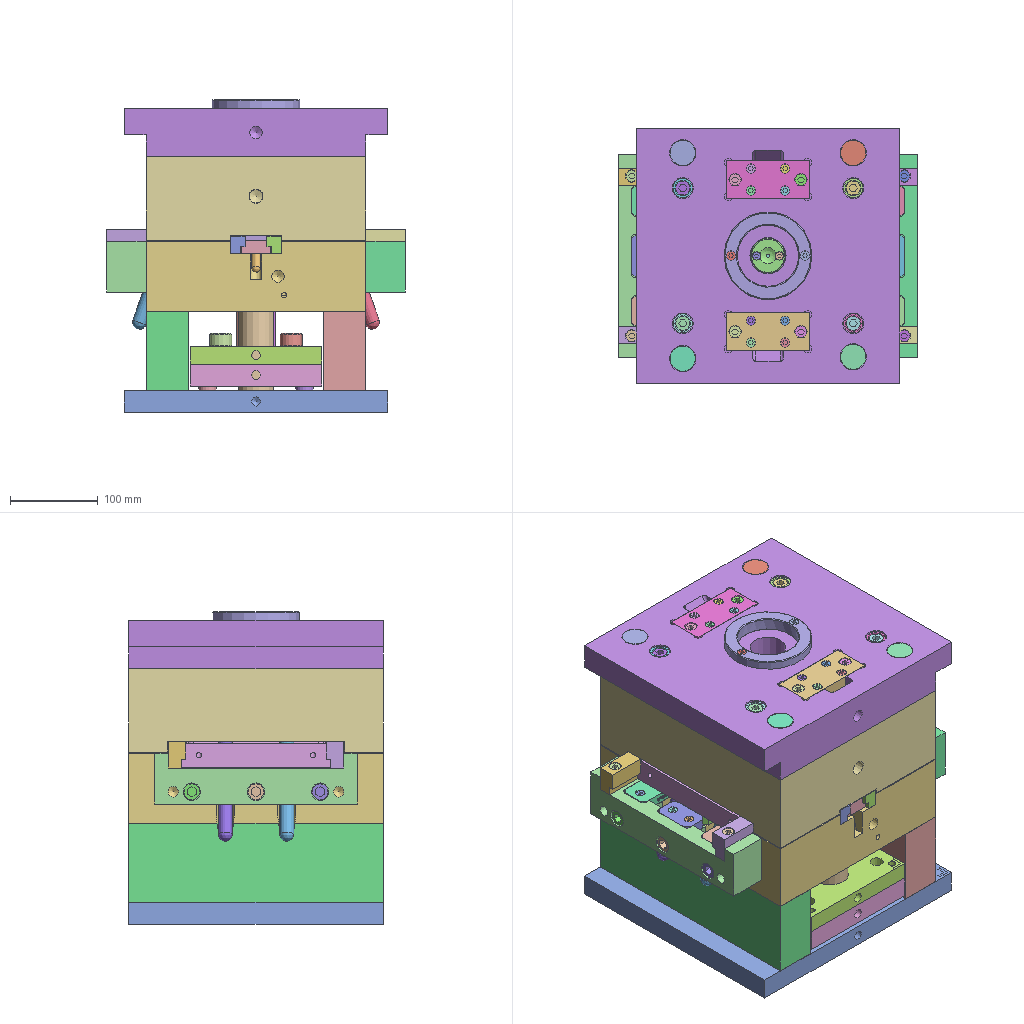Assembly | STEP file | 210 different items | 210 placed | box 340 x 290 x 356 mm
Parts list (item | name | quantity | parent item | size | volume):
1 | AA_id278_x_t | x1 | in lll_x_t | 250 x 290 x 95 mm | 4489597 mm3
2 | AD_id274_x_t | x1 | in lll_x_t | 300 x 290 x 55 mm | 3688496 mm3
3 | BB_id58_x_t | x1 | in lll_x_t | 250 x 290 x 80 mm | 3575390 mm3
4 | BD_id262_x_t | x1 | in lll_x_t | 300 x 290 x 25 mm | 2072800 mm3
5 | CC01_id270_x_t | x1 | in lll_x_t | 48 x 290 x 90 mm | 1057434 mm3
6 | CC02_id266_x_t | x1 | in lll_x_t | 48 x 290 x 90 mm | 1057434 mm3
7 | DDZ6.00_id214_x_t | x1 | in lll_x_t | 10 x 10 x 160.68 mm | 4845 mm3
8 | DDZ6.00_id218_x_t | x1 | in lll_x_t | 10 x 10 x 160.68 mm | 4845 mm3
9 | DDZ6.00_id222_x_t | x1 | in lll_x_t | 10 x 10 x 160.68 mm | 4845 mm3
10 | DDZ6.00_id226_x_t | x1 | in lll_x_t | 10 x 10 x 160.68 mm | 4845 mm3
11 | DDZ6.00_id234_x_t | x1 | in lll_x_t | 10 x 10 x 160.68 mm | 4845 mm3
12 | DDZ6.00_id238_x_t | x1 | in lll_x_t | 10 x 10 x 160.68 mm | 4845 mm3
13 | DDZ6.00_id242_x_t | x1 | in lll_x_t | 10 x 10 x 160.68 mm | 4845 mm3
14 | DDZ6.00_id246_x_t | x1 | in lll_x_t | 10 x 10 x 160.68 mm | 4845 mm3
15 | DDZ6.00_id250_x_t | x1 | in lll_x_t | 10 x 10 x 166.5 mm | 5009 mm3
16 | DDZ6.00_id50_x_t | x1 | in lll_x_t | 10 x 10 x 166.5 mm | 2539 mm3
17 | DDZ6.00_id54_x_t | x1 | in lll_x_t | 10 x 10 x 166.5 mm | 2539 mm3
18 | DDZ8.00_id210_x_t | x1 | in lll_x_t | 13 x 13 x 135.432 mm | 4709 mm3
19 | DZDB_id254_x_t | x1 | in lll_x_t | 150 x 290 x 25 mm | 967966 mm3
20 | DZMB_id258_x_t | x1 | in lll_x_t | 150 x 290 x 20 mm | 774159 mm3
21 | LJD_id162_x_t | x1 | in lll_x_t | 12 x 12 x 15 mm | 521.973 mm3
22 | LJD_id166_x_t | x1 | in lll_x_t | 20 x 20 x 5 mm | 1219 mm3
23 | LJD_id170_x_t | x1 | in lll_x_t | 12 x 12 x 15 mm | 521.973 mm3
24 | LJD_id174_x_t | x1 | in lll_x_t | 20 x 20 x 5 mm | 1219 mm3
25 | LJD_id178_x_t | x1 | in lll_x_t | 12 x 12 x 15 mm | 521.973 mm3
26 | LJD_id182_x_t | x1 | in lll_x_t | 20 x 20 x 5 mm | 1219 mm3
27 | LJD_id186_x_t | x1 | in lll_x_t | 12 x 12 x 15 mm | 521.973 mm3
28 | LJD_id190_x_t | x1 | in lll_x_t | 20 x 20 x 5 mm | 1219 mm3
29 | LJD_id194_x_t | x1 | in lll_x_t | 12 x 12 x 15 mm | 521.973 mm3
30 | LJD_id198_x_t | x1 | in lll_x_t | 20 x 20 x 5 mm | 1219 mm3
31 | LJD_id202_x_t | x1 | in lll_x_t | 12 x 12 x 15 mm | 521.973 mm3
32 | LJD_id206_x_t | x1 | in lll_x_t | 20 x 20 x 5 mm | 1219 mm3
33 | M6.00-20.00_id118_x_t | x1 | in lll_x_t | 10 x 10 x 29 mm | 1051 mm3
34 | M6.00-20.00_id126_x_t | x1 | in lll_x_t | 10 x 10 x 29 mm | 1051 mm3
35 | M6.00-20.00_id134_x_t | x1 | in lll_x_t | 10 x 10 x 29 mm | 1051 mm3
36 | M6.00-20.00_id142_x_t | x1 | in lll_x_t | 10 x 10 x 29 mm | 1051 mm3
37 | lll_id102_x_t | x1 | in lll_x_t | 25 x 52.484 x 63.172 mm | 22828 mm3
38 | lll_id106_x_t | x1 | in lll_x_t | 90 x 160 x 68.59 mm | 417542 mm3
39 | lll_id10_x_t | x1 | in lll_x_t | 62 x 18 x 18 mm | 8023 mm3
40 | lll_id110_x_t | x1 | in lll_x_t | 40 x 40 x 90 mm | 111990 mm3
41 | lll_id114_x_t | x1 | in lll_x_t | 40 x 40 x 90 mm | 111990 mm3
42 | lll_id122_x_t | x1 | in lll_x_t | 25 x 25 x 15 mm | 6356 mm3
43 | lll_id130_x_t | x1 | in lll_x_t | 25 x 25 x 15 mm | 6356 mm3
44 | lll_id138_x_t | x1 | in lll_x_t | 25 x 25 x 15 mm | 6356 mm3
45 | lll_id146_x_t | x1 | in lll_x_t | 25 x 25 x 15 mm | 6356 mm3
46 | lll_id14_x_t | x1 | in lll_x_t | 62 x 18 x 18 mm | 8023 mm3
47 | lll_id150_x_t | x1 | in lll_x_t | 41 x 46 x 48 mm | 57755 mm3
48 | lll_id154_x_t | x1 | in lll_x_t | 40 x 40 x 59.5 mm | 20901 mm3
49 | lll_id158_x_t | x1 | in lll_x_t | 99.8 x 99.8 x 15 mm | 57338 mm3
50 | lll_id18_x_t | x1 | in lll_x_t | 62 x 18 x 18 mm | 8023 mm3
51 | lll_id22_x_t | x1 | in lll_x_t | 62 x 18 x 18 mm | 8023 mm3
52 | lll_id230_x_t | x1 | in lll_x_t | 38.894 x 25.019 x 83.75 mm | 50062 mm3
53 | lll_id26_x_t | x1 | in lll_x_t | 62 x 18 x 18 mm | 8023 mm3
54 | lll_id282_x_t | x1 | in lll_x_t | 22 x 22 x 59 mm | 7367 mm3
55 | lll_id286_x_t | x1 | in lll_x_t | 15 x 32.483 x 61.146 mm | 5638 mm3
56 | lll_id290_x_t | x1 | in lll_x_t | 17 x 31 x 10 mm | 3483 mm3
57 | lll_id294_x_t | x1 | in lll_x_t | 10 x 10 x 10 mm | 477.247 mm3
58 | lll_id298_x_t | x1 | in lll_x_t | 50 x 29 x 25 mm | 24612 mm3
59 | lll_id302_x_t | x1 | in lll_x_t | 16 x 60 x 20 mm | 14663 mm3
60 | lll_id306_x_t | x1 | in lll_x_t | 16 x 60 x 20 mm | 14663 mm3
61 | lll_id30_x_t | x1 | in lll_x_t | 10 x 53.41 x 81.544 mm | 2497 mm3
62 | lll_id310_x_t | x1 | in lll_x_t | 81.68 x 20 x 184.615 mm | 39750 mm3
63 | lll_id314_x_t | x1 | in lll_x_t | 35 x 52 x 12 mm | 19640 mm3
64 | lll_id318_x_t | x1 | in lll_x_t | 81.68 x 20 x 184.615 mm | 39750 mm3
65 | lll_id322_x_t | x1 | in lll_x_t | 35 x 52 x 12 mm | 19640 mm3
66 | lll_id326_x_t | x1 | in lll_x_t | 50 x 29 x 25 mm | 24612 mm3
67 | lll_id330_x_t | x1 | in lll_x_t | 15 x 32.483 x 61.146 mm | 5638 mm3
68 | lll_id334_x_t | x1 | in lll_x_t | 10 x 10 x 10 mm | 477.247 mm3
69 | lll_id338_x_t | x1 | in lll_x_t | 17 x 31 x 10 mm | 3483 mm3
70 | lll_id342_x_t | x1 | in lll_x_t | 16 x 60 x 20 mm | 14663 mm3
71 | lll_id346_x_t | x1 | in lll_x_t | 16 x 60 x 20 mm | 14663 mm3
72 | lll_id34_x_t | x1 | in lll_x_t | 25 x 52.484 x 63.172 mm | 22828 mm3
73 | lll_id350_x_t | x1 | in lll_x_t | 35 x 52 x 12 mm | 19640 mm3
74 | lll_id354_x_t | x1 | in lll_x_t | 45 x 230 x 58 mm | 337405 mm3
75 | lll_id358_x_t | x1 | in lll_x_t | 140 x 20 x 30 mm | 68147 mm3
76 | lll_id362_x_t | x1 | in lll_x_t | 140 x 20 x 30 mm | 68146 mm3
77 | lll_id366_x_t | x1 | in lll_x_t | 30 x 50 x 12 mm | 15790 mm3
78 | lll_id370_x_t | x1 | in lll_x_t | 60 x 35 x 12 mm | 22990 mm3
79 | lll_id374_x_t | x1 | in lll_x_t | 60 x 35 x 12 mm | 22990 mm3
80 | lll_id378_x_t | x1 | in lll_x_t | 30 x 50 x 12 mm | 15790 mm3
81 | lll_id382_x_t | x1 | in lll_x_t | 20 x 30 x 23 mm | 8328 mm3
82 | lll_id386_x_t | x1 | in lll_x_t | 20 x 30 x 23 mm | 8328 mm3
83 | lll_id38_x_t | x1 | in lll_x_t | 34 x 86.656 x 30 mm | 42409 mm3
84 | lll_id390_x_t | x1 | in lll_x_t | 50 x 80 x 12 mm | 42551 mm3
85 | lll_id394_x_t | x1 | in lll_x_t | 50 x 80 x 12 mm | 42551 mm3
86 | lll_id398_x_t | x1 | in lll_x_t | 50 x 80 x 12 mm | 42551 mm3
87 | lll_id402_x_t | x1 | in lll_x_t | 20 x 30 x 23 mm | 8328 mm3
88 | lll_id406_x_t | x1 | in lll_x_t | 20 x 30 x 23 mm | 8328 mm3
89 | lll_id410_x_t | x1 | in lll_x_t | 140 x 20 x 30 mm | 68147 mm3
90 | lll_id414_x_t | x1 | in lll_x_t | 140 x 20 x 30 mm | 68146 mm3
91 | lll_id418_x_t | x1 | in lll_x_t | 38.894 x 25.019 x 83.75 mm | 50059 mm3
92 | lll_id422_x_t | x1 | in lll_x_t | 50 x 80 x 12 mm | 42551 mm3
93 | lll_id426_x_t | x1 | in lll_x_t | 30 x 50 x 12 mm | 15790 mm3
94 | lll_id42_x_t | x1 | in lll_x_t | 10 x 53.41 x 81.544 mm | 2497 mm3
95 | lll_id430_x_t | x1 | in lll_x_t | 30 x 50 x 12 mm | 15790 mm3
96 | lll_id434_x_t | x1 | in lll_x_t | 60 x 35 x 12 mm | 22990 mm3
97 | lll_id438_x_t | x1 | in lll_x_t | 60 x 35 x 12 mm | 22990 mm3
98 | lll_id442_x_t | x1 | in lll_x_t | 29.857 x 70 x 50.854 mm | 39790 mm3
99 | lll_id446_x_t | x1 | in lll_x_t | 29.857 x 70 x 50.854 mm | 39790 mm3
100 | lll_id450_x_t | x1 | in lll_x_t | 81.68 x 20 x 184.615 mm | 39750 mm3
101 | lll_id454_x_t | x1 | in lll_x_t | 35 x 52 x 12 mm | 19640 mm3
102 | lll_id458_x_t | x1 | in lll_x_t | 45 x 230 x 58 mm | 337405 mm3
103 | lll_id462_x_t | x1 | in lll_x_t | 81.68 x 20 x 184.615 mm | 39750 mm3
104 | lll_id466_x_t | x1 | in lll_x_t | 29.857 x 70 x 50.854 mm | 39790 mm3
105 | lll_id46_x_t | x1 | in lll_x_t | 55.309 x 41.141 x 59.468 mm | 14807 mm3
106 | lll_id470_x_t | x1 | in lll_x_t | 29.857 x 70 x 50.854 mm | 39790 mm3
107 | lll_id474_x_t | x1 | in lll_x_t | 95 x 43 x 18 mm | 65617 mm3
108 | lll_id478_x_t | x1 | in lll_x_t | 55 x 43 x 38 mm | 62976 mm3
109 | lll_id482_x_t | x1 | in lll_x_t | 10 x 10 x 21 mm | 809.617 mm3
110 | lll_id486_x_t | x1 | in lll_x_t | 10 x 10 x 21 mm | 809.617 mm3
111 | lll_id490_x_t | x1 | in lll_x_t | 10 x 10 x 21 mm | 809.617 mm3
112 | lll_id494_x_t | x1 | in lll_x_t | 10 x 10 x 21 mm | 809.617 mm3
113 | lll_id498_x_t | x1 | in lll_x_t | 10 x 10 x 21 mm | 809.617 mm3
114 | lll_id502_x_t | x1 | in lll_x_t | 10 x 10 x 21 mm | 809.617 mm3
115 | lll_id506_x_t | x1 | in lll_x_t | 13 x 13 x 23 mm | 1651 mm3
116 | lll_id510_x_t | x1 | in lll_x_t | 13 x 13 x 23 mm | 1651 mm3
117 | lll_id514_x_t | x1 | in lll_x_t | 8.5 x 8.5 x 15 mm | 434.348 mm3
118 | lll_id518_x_t | x1 | in lll_x_t | 8.5 x 8.5 x 15 mm | 434.348 mm3
119 | lll_id522_x_t | x1 | in lll_x_t | 29 x 29 x 271 mm | 134679 mm3
120 | lll_id526_x_t | x1 | in lll_x_t | 13 x 13 x 23 mm | 1651 mm3
121 | lll_id530_x_t | x1 | in lll_x_t | 13 x 13 x 23 mm | 1651 mm3
122 | lll_id534_x_t | x1 | in lll_x_t | 10 x 10 x 21 mm | 809.617 mm3
123 | lll_id538_x_t | x1 | in lll_x_t | 10 x 10 x 21 mm | 809.617 mm3
124 | lll_id542_x_t | x1 | in lll_x_t | 10 x 10 x 21 mm | 809.617 mm3
125 | lll_id546_x_t | x1 | in lll_x_t | 10 x 10 x 21 mm | 809.617 mm3
126 | lll_id550_x_t | x1 | in lll_x_t | 95 x 43 x 18 mm | 65617 mm3
127 | lll_id554_x_t | x1 | in lll_x_t | 22 x 22 x 59 mm | 7367 mm3
128 | lll_id558_x_t | x1 | in lll_x_t | 22 x 22 x 59 mm | 7367 mm3
129 | lll_id562_x_t | x1 | in lll_x_t | 22 x 22 x 59 mm | 7367 mm3
130 | lll_id566_x_t | x1 | in lll_x_t | 29 x 29 x 271 mm | 134679 mm3
131 | lll_id570_x_t | x1 | in lll_x_t | 29 x 29 x 271 mm | 134679 mm3
132 | lll_id574_x_t | x1 | in lll_x_t | 29 x 29 x 271 mm | 134679 mm3
133 | lll_id578_x_t | x1 | in lll_x_t | 38 x 38 x 67 mm | 32777 mm3
134 | lll_id582_x_t | x1 | in lll_x_t | 38 x 38 x 67 mm | 32777 mm3
135 | lll_id586_x_t | x1 | in lll_x_t | 38 x 38 x 67 mm | 32777 mm3
136 | lll_id590_x_t | x1 | in lll_x_t | 38 x 38 x 67 mm | 32777 mm3
137 | lll_id594_x_t | x1 | in lll_x_t | 10 x 10 x 16 mm | 668.246 mm3
138 | lll_id598_x_t | x1 | in lll_x_t | 10 x 10 x 16 mm | 668.246 mm3
139 | lll_id602_x_t | x1 | in lll_x_t | 10 x 10 x 16 mm | 668.246 mm3
140 | lll_id606_x_t | x1 | in lll_x_t | 10 x 10 x 16 mm | 668.246 mm3
141 | lll_id610_x_t | x1 | in lll_x_t | 10 x 10 x 16 mm | 668.246 mm3
142 | lll_id614_x_t | x1 | in lll_x_t | 10 x 10 x 16 mm | 668.246 mm3
143 | lll_id618_x_t | x1 | in lll_x_t | 10 x 10 x 16 mm | 668.246 mm3
144 | lll_id622_x_t | x1 | in lll_x_t | 10 x 10 x 16 mm | 668.246 mm3
145 | lll_id626_x_t | x1 | in lll_x_t | 16 x 16 x 70 mm | 6357 mm3
146 | lll_id62_x_t | x1 | in lll_x_t | 51.763 x 39.033 x 66.18 mm | 50853 mm3
147 | lll_id630_x_t | x1 | in lll_x_t | 16 x 16 x 70 mm | 6357 mm3
148 | lll_id634_x_t | x1 | in lll_x_t | 16 x 16 x 70 mm | 6357 mm3
149 | lll_id638_x_t | x1 | in lll_x_t | 16 x 16 x 70 mm | 6357 mm3
150 | lll_id642_x_t | x1 | in lll_x_t | 30 x 30 x 20 mm | 11962 mm3
151 | lll_id646_x_t | x1 | in lll_x_t | 30 x 30 x 20 mm | 11962 mm3
152 | lll_id650_x_t | x1 | in lll_x_t | 30 x 30 x 20 mm | 11962 mm3
153 | lll_id654_x_t | x1 | in lll_x_t | 17.832 x 10 x 13.411 mm | 668.246 mm3
154 | lll_id658_x_t | x1 | in lll_x_t | 17.832 x 10 x 13.411 mm | 668.246 mm3
155 | lll_id662_x_t | x1 | in lll_x_t | 17.832 x 10 x 13.411 mm | 668.246 mm3
156 | lll_id666_x_t | x1 | in lll_x_t | 17.832 x 10 x 13.411 mm | 668.246 mm3
157 | lll_id66_x_t | x1 | in lll_x_t | 10 x 10 x 41 mm | 1392 mm3
158 | lll_id670_x_t | x1 | in lll_x_t | 17.832 x 10 x 13.411 mm | 668.246 mm3
159 | lll_id674_x_t | x1 | in lll_x_t | 17.832 x 10 x 13.411 mm | 668.246 mm3
160 | lll_id678_x_t | x1 | in lll_x_t | 17.832 x 10 x 13.411 mm | 668.246 mm3
161 | lll_id682_x_t | x1 | in lll_x_t | 17.832 x 10 x 13.411 mm | 668.246 mm3
162 | lll_id686_x_t | x1 | in lll_x_t | 13 x 13 x 33 mm | 2154 mm3
163 | lll_id690_x_t | x1 | in lll_x_t | 13 x 13 x 33 mm | 2154 mm3
164 | lll_id694_x_t | x1 | in lll_x_t | 13 x 13 x 33 mm | 2154 mm3
165 | lll_id698_x_t | x1 | in lll_x_t | 13 x 13 x 33 mm | 2154 mm3
166 | lll_id6_x_t | x1 | in lll_x_t | 62 x 18 x 18 mm | 8023 mm3
167 | lll_id702_x_t | x1 | in lll_x_t | 13 x 13 x 33 mm | 2154 mm3
168 | lll_id706_x_t | x1 | in lll_x_t | 13 x 13 x 33 mm | 2154 mm3
169 | lll_id70_x_t | x1 | in lll_x_t | 10 x 10 x 41 mm | 1392 mm3
170 | lll_id710_x_t | x1 | in lll_x_t | 13 x 13 x 33 mm | 2154 mm3
171 | lll_id714_x_t | x1 | in lll_x_t | 13 x 13 x 33 mm | 2154 mm3
172 | lll_id718_x_t | x1 | in lll_x_t | 10 x 10 x 26 mm | 950.989 mm3
173 | lll_id722_x_t | x1 | in lll_x_t | 10 x 10 x 26 mm | 950.989 mm3
174 | lll_id726_x_t | x1 | in lll_x_t | 10 x 10 x 26 mm | 950.989 mm3
175 | lll_id730_x_t | x1 | in lll_x_t | 10 x 10 x 26 mm | 950.989 mm3
176 | lll_id734_x_t | x1 | in lll_x_t | 10 x 10 x 26 mm | 950.989 mm3
177 | lll_id738_x_t | x1 | in lll_x_t | 10 x 10 x 26 mm | 950.989 mm3
178 | lll_id742_x_t | x1 | in lll_x_t | 10 x 10 x 26 mm | 950.989 mm3
179 | lll_id746_x_t | x1 | in lll_x_t | 10 x 10 x 26 mm | 950.989 mm3
180 | lll_id74_x_t | x1 | in lll_x_t | 10 x 10 x 41 mm | 1392 mm3
181 | lll_id750_x_t | x1 | in lll_x_t | 10 x 10 x 18 mm | 724.794 mm3
182 | lll_id754_x_t | x1 | in lll_x_t | 10 x 10 x 18 mm | 724.794 mm3
183 | lll_id758_x_t | x1 | in lll_x_t | 10 x 10 x 18 mm | 724.794 mm3
184 | lll_id762_x_t | x1 | in lll_x_t | 10 x 10 x 18 mm | 724.794 mm3
185 | lll_id766_x_t | x1 | in lll_x_t | 10 x 10 x 18 mm | 724.794 mm3
186 | lll_id770_x_t | x1 | in lll_x_t | 10 x 10 x 18 mm | 724.794 mm3
187 | lll_id774_x_t | x1 | in lll_x_t | 10 x 10 x 18 mm | 724.794 mm3
188 | lll_id778_x_t | x1 | in lll_x_t | 10 x 10 x 18 mm | 724.794 mm3
189 | lll_id782_x_t | x1 | in lll_x_t | 10 x 10 x 18 mm | 724.794 mm3
190 | lll_id786_x_t | x1 | in lll_x_t | 10 x 10 x 18 mm | 724.794 mm3
191 | lll_id78_x_t | x1 | in lll_x_t | 10 x 10 x 41 mm | 1392 mm3
192 | lll_id790_x_t | x1 | in lll_x_t | 10 x 10 x 18 mm | 724.794 mm3
193 | lll_id794_x_t | x1 | in lll_x_t | 10 x 10 x 18 mm | 724.794 mm3
194 | lll_id798_x_t | x1 | in lll_x_t | 10 x 10 x 18 mm | 724.794 mm3
195 | lll_id802_x_t | x1 | in lll_x_t | 10 x 10 x 18 mm | 724.794 mm3
196 | lll_id806_x_t | x1 | in lll_x_t | 10 x 10 x 18 mm | 724.794 mm3
197 | lll_id810_x_t | x1 | in lll_x_t | 10 x 10 x 18 mm | 724.794 mm3
198 | lll_id814_x_t | x1 | in lll_x_t | 10 x 10 x 18 mm | 724.794 mm3
199 | lll_id818_x_t | x1 | in lll_x_t | 10 x 10 x 18 mm | 724.794 mm3
200 | lll_id822_x_t | x1 | in lll_x_t | 10 x 10 x 18 mm | 724.794 mm3
201 | lll_id826_x_t | x1 | in lll_x_t | 10 x 10 x 18 mm | 724.794 mm3
202 | lll_id82_x_t | x1 | in lll_x_t | 51.763 x 39.033 x 66.18 mm | 54885 mm3
203 | lll_id830_x_t | x1 | in lll_x_t | 10 x 10 x 18 mm | 724.794 mm3
204 | lll_id834_x_t | x1 | in lll_x_t | 10 x 10 x 18 mm | 724.794 mm3
205 | lll_id838_x_t | x1 | in lll_x_t | 10 x 10 x 18 mm | 724.794 mm3
206 | lll_id842_x_t | x1 | in lll_x_t | 10 x 10 x 18 mm | 724.794 mm3
207 | lll_id86_x_t | x1 | in lll_x_t | 130 x 169 x 80 mm | 855634 mm3
208 | lll_id90_x_t | x1 | in lll_x_t | 125 x 169 x 80 mm | 846021 mm3
209 | lll_id94_x_t | x1 | in lll_x_t | 30 x 30 x 20 mm | 11962 mm3
210 | lll_id98_x_t | x1 | in lll_x_t | 34 x 86.656 x 30 mm | 42409 mm3